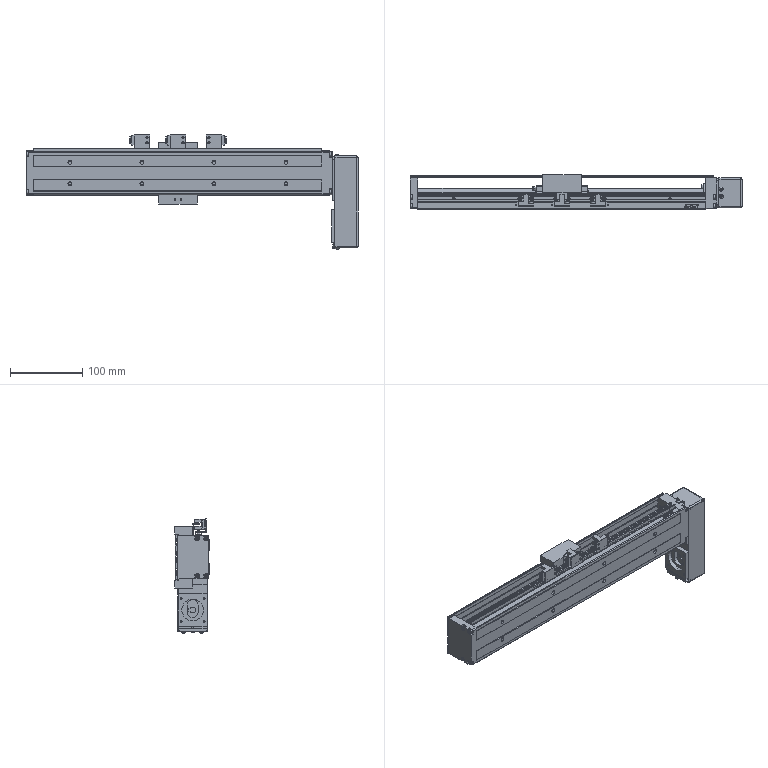Part | SolidWorks | 7 solids | 1773 faces | box 461 x 48 x 158.3 mm | volume 640236 mm3 | plane 1040 | cylinder 413 | spline 202 | cone 116 | torus 2 | commonest cylinder face diameters 1 x80 5.5 x72 3 x56 2.113 x24 9.5 x24 6 x22